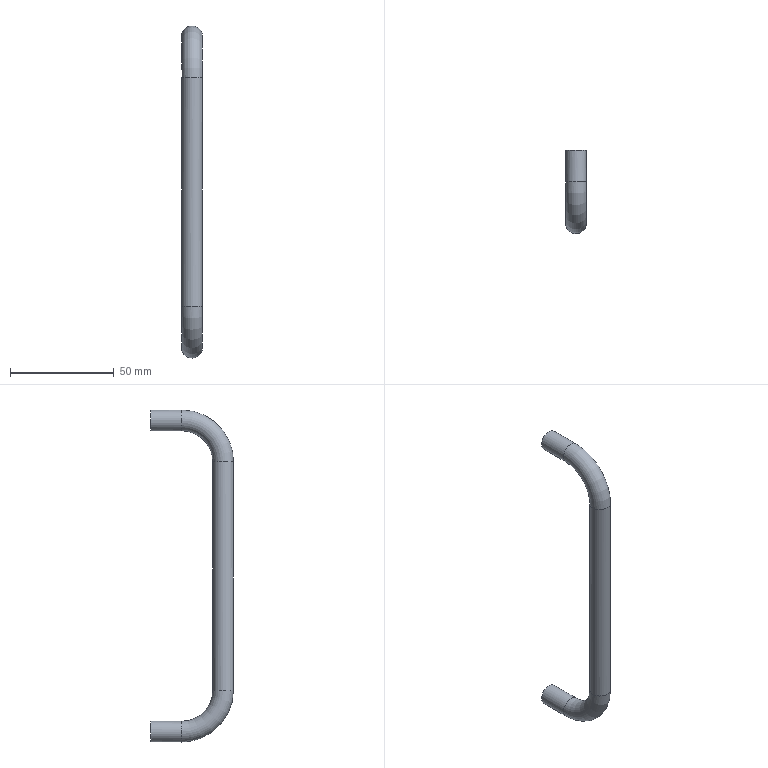Part | STEP file | SOLID | 1 solid | 13 faces | box 10 x 40 x 160 mm | volume 15544 mm3 | cylinder 5 | cone 4 | plane 2 | torus 2 | commonest cylinder face diameters 10 x3 4.2 x2